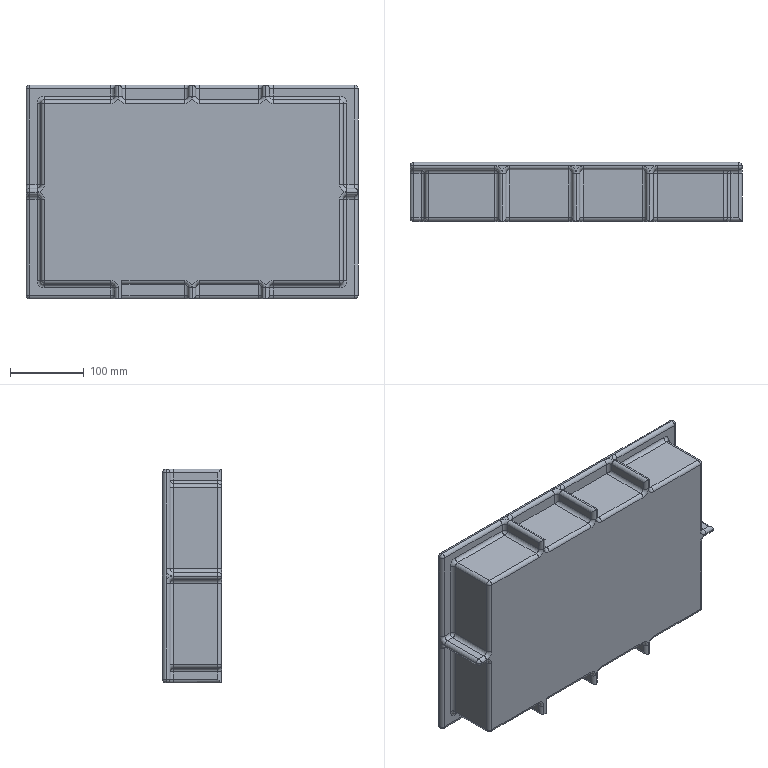Part | STEP file | Basket 1 | 1 solid | 215 faces | box 450 x 80 x 290 mm | volume 2294003 mm3 | cylinder 108 | plane 51 | torus 34 | sphere 22 | commonest cylinder face diameters 10 x108